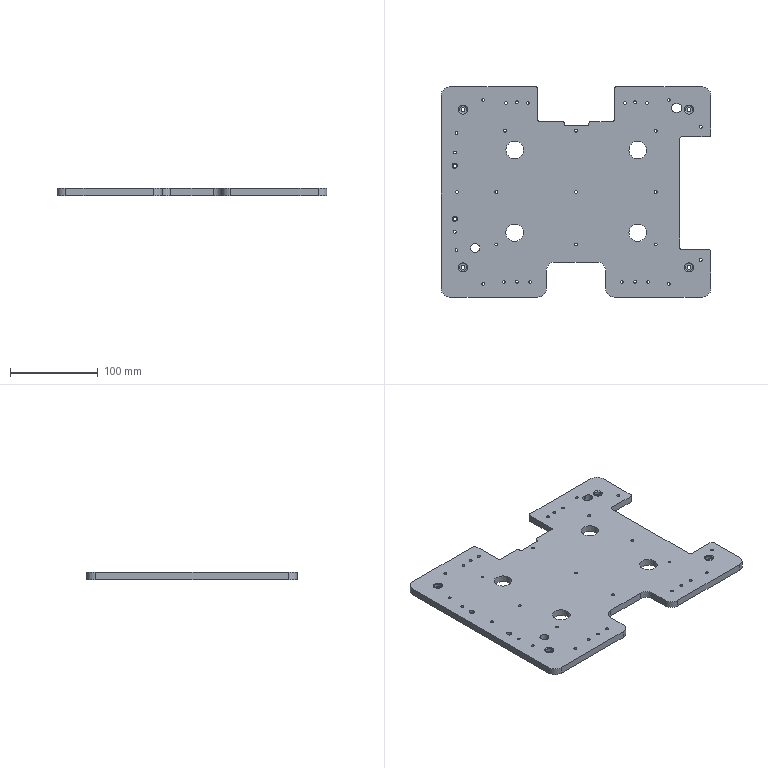CAM job | NX | 3-axis milling, drilling | part box 308 x 240 x 8 mm | stock box 313 x 245 x 8 mm
Tools:
number,name,description,diameter,corner_radius,flute_length,length,flutes
4,D4,平底铣刀-粗,4.0,0.0,25.0,75.0,2
6,D6,平底铣刀-粗,6.0,0.0,25.0,75.0,2
9,D10,平底铣刀-粗,10.0,0.0,35.0,75.0,2
18,D4-J,平底铣刀-精,4.0,0.0,50.0,75.0,2
7,D6-J,平底铣刀-精,6.0,0.0,25.0,75.0,2
10,D10-J,平底铣刀-精,10.0,0.0,35.0,75.0,2
2,D6_CHAMFER_TOOL,倒角刀,6.0,0.0,3.0,25.0,2
21,M4X0.7,丝锥,3.3,0.0,35.0,50.0,2
17,ZT4,钻头,4.0,0.0,35.0,50.0,2
11,ZT4.5,钻头,4.5,0.0,35.0,50.0,2
13,DRILL_BIT_3.3,Twist Drill 3.3 mm,3.3,0.0,35.0,35.008,2
Operations:
program,operation,operation_type,tool,method,geometry_group,spindle_rpm,surface_speed,feed_per_tooth,feed_cut,feed_plunge,cut_length_mm,path_length_mm,cut_time_min,machine_time_min
B,SPOT-DEPTH0.8,Operation,D6_CHAMFER_TOOL,NONE,W-B,8000.0,150.796,0.0312,500.0,90.0,75.6,1504.572,0.1512,0.2941
B,SPOT0.8,Operation,D6_CHAMFER_TOOL,METHOD,W-B,8000.0,150.796,0.0312,500.0,0.0,1.8,43.6,0.0036,0.0078
B,THROUGH_HOLE-M4_TAP_DRILL,Operation,DRILL_BIT_3.3,NONE,W-B,3000.0,31.102,0.05,300.0,90.0,479.725,2213.567,1.599,1.772
B,THROUGH_HOLE-4.0_PRECISION_PRE-DRILL,Operation,ZT4,NONE,W-B,3000.0,36.757,0.0417,250.0,90.0,20.403,142.495,0.0816,0.0938
B,THROUGH_HOLE-5-6,Operation,ZT4.5,NONE,W-B,3000.0,42.411,0.025,150.0,90.0,31.408,723.823,0.2094,0.2786
B,C0.3_CLOSED_CONTOUR_CHAMFER6X45L_COPY,PlanarMilling,D6_CHAMFER_TOOL,WALL_CHAMFER-DEPTH0-STEPG,W-B,7000.0,131.0,0.1071,1500.0,100.0,1636.563,2327.985,1.091,1.16
B,C0.3_CLOSED_CONTOUR_CHAMFER6X45L_COPY_1,PlanarMilling,D6_CHAMFER_TOOL,WALL_CHAMFER-DEPTH0-STEPG,W-B,7000.0,131.0,0.1071,1500.0,100.0,44.251,80.251,0.0295,0.0331
B,DRILL_CHAMFER_2,Operation,D6_CHAMFER_TOOL,METHOD,W-B,8000.0,150.796,0.0312,500.0,0.0,166.4,1653.496,0.3328,0.4815
B,DRILL_CHAMFER_3,Operation,D6_CHAMFER_TOOL,METHOD,W-B,8000.0,150.796,0.0312,500.0,0.0,10.6,124.954,0.0212,0.0326
B,MILL_CHAMFER_4,PlanarMilling,D6_CHAMFER_TOOL,METHOD,W-B,8000.0,150.796,0.0312,500.0,100.0,69.412,850.315,0.1388,0.2169
B,THROUGH_HOLE-TAP_M4,Operation,M4X0.7,METHOD,W-B,600.0,6.22,0.0006,0.7,90.0,384.0,2022.116,548.571,548.735
A,SPOT,Operation,D6_CHAMFER_TOOL,METHOD,W-A,3000.0,56.549,0.0333,200.0,0.0,107.5,1596.228,0.5375,0.6864
A,DRILL_HOLE_2,Operation,ZT4,METHOD,W-A,3000.0,37.699,0.02,120.0,0.0,17.4,136.488,0.145,0.1569
A,DRILL_HOLE_3,Operation,ZT4.5,METHOD,W-A,2500.0,35.343,0.024,120.0,0.0,34.8,730.607,0.29,0.3596
A,HOLE_ROUGH_4,CylinderMilling,D10,METHOD,W-A,6000.0,157.0,0.25,3000.0,90.0,4554.584,5073.221,1.519,1.571
A,OUTLINE_ROUGH_2,VolumeBased25DMillingOperation,D10,METHOD,W-A,6000.0,188.0,0.25,4000.0,80.0,23680.739,23726.739,5.92,5.925
A,THROUGH_WAIST_SLOT_ROUGH_1,VolumeBased25DMillingOperation,D6,METHOD,W-A,8000.0,150.796,0.0375,600.0,100.0,911.661,957.858,1.519,1.524
A,FLOOR_WALL_HELIX_ROUGH-MID_COPY,VolumeBased25DMillingOperation,D6,LEVEL_ROUGH-DEPTHK-STEPG,W-A,8000.0,150.796,0.0375,600.0,100.0,234.283,279.98,0.3905,0.395
A,HOLE_ROUGH_1,CylinderMilling,D4,METHOD,W-A,6000.0,75.398,0.1,1200.0,100.0,216.126,362.206,0.1801,0.1947
A,HOLE_ROUGH_2,CylinderMilling,D4,METHOD,W-A,6000.0,75.398,0.15,1800.0,100.0,990.419,1781.219,0.5502,0.6293
A,HOLE_SIDE_4,CylinderMilling,D10-J,METHOD,W-A,6000.0,157.0,0.0833,1000.0,90.0,175.257,726.992,0.1779,0.2331
A,OUTLINE_D4_CORNER_CLEAN,ZLevelMilling,D4-J,METHOD,W-A,6000.0,75.0,0.25,2500.0,80.0,1105.119,1642.302,0.4426,0.4963
A,CHAMFER_2,SurfaceContour,D6_CHAMFER_TOOL,METHOD,W-A,6000.0,113.0,0.125,1200.0,100.0,1599.691,2304.978,1.333,1.404
A,DRILL_CHAMFER_1,Operation,D6_CHAMFER_TOOL,METHOD,W-A,5000.0,94.248,0.015,150.0,0.0,166.4,1653.496,1.109,1.258
A,MILL_CHAMFER_1,PlanarMilling,D6_CHAMFER_TOOL,METHOD,W-A,6000.0,113.097,0.05,600.0,100.0,23.913,171.219,0.0399,0.0546
A,MILL_CHAMFER_2,PlanarMilling,D6_CHAMFER_TOOL,METHOD,W-A,6000.0,113.097,0.05,600.0,100.0,138.685,924.741,0.2311,0.3097
A,MILL_CHAMFER_3,PlanarMilling,D6_CHAMFER_TOOL,METHOD,W-A,6000.0,113.097,0.05,600.0,100.0,31.489,75.089,0.0525,0.0568
A,WAIST_SLOT_FINISH_1,VolumeBased25DMillingOperation,D6-J,METHOD,W-A,6000.0,113.0,0.025,300.0,100.0,68.102,475.989,0.227,0.2678
A,FLOOR_WALL_FINISH_SIDE-MID-SELECT_FLOOR_COPY,VolumeBased25DMillingOperation,D4-J,SIDE_FINISH-DEPTHK-STEPG,W-A,8000.0,100.531,0.0312,500.0,100.0,105.191,895.828,0.2104,0.2894
A,OUTLINE_SEMI_FINISH_2,VolumeBased25DMillingOperation,D6-J,METHOD,W-A,6000.0,113.0,0.0833,1000.0,100.0,1311.973,1365.973,1.312,1.317
A,OUTLINE_FINISH_2,VolumeBased25DMillingOperation,D6-J,METHOD,W-A,6000.0,113.0,0.0833,1000.0,100.0,1311.773,1366.373,1.312,1.317